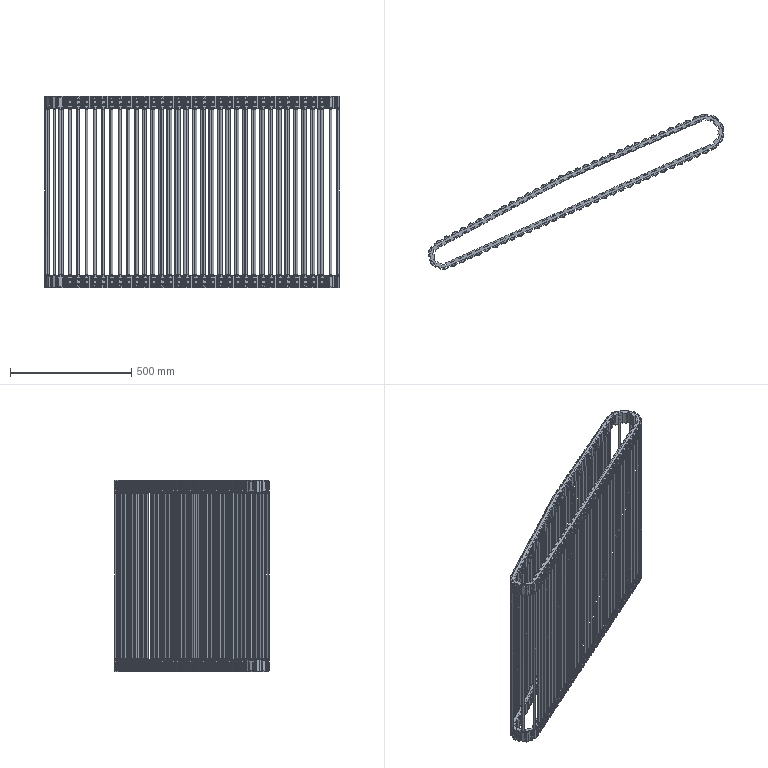Part | SolidWorks | features ReferencePattern 399, CompositeCurve 20, LocalLPattern 6 | 451 solids | 41462 faces | volume 9156877 mm3 | cone 30744 | plane 6714 | cylinder 3074 | torus 930 | commonest cylinder face diameters 4 x1072 3.3 x504 3.464 x504 8.4 x504 18.167 x284 10 x142